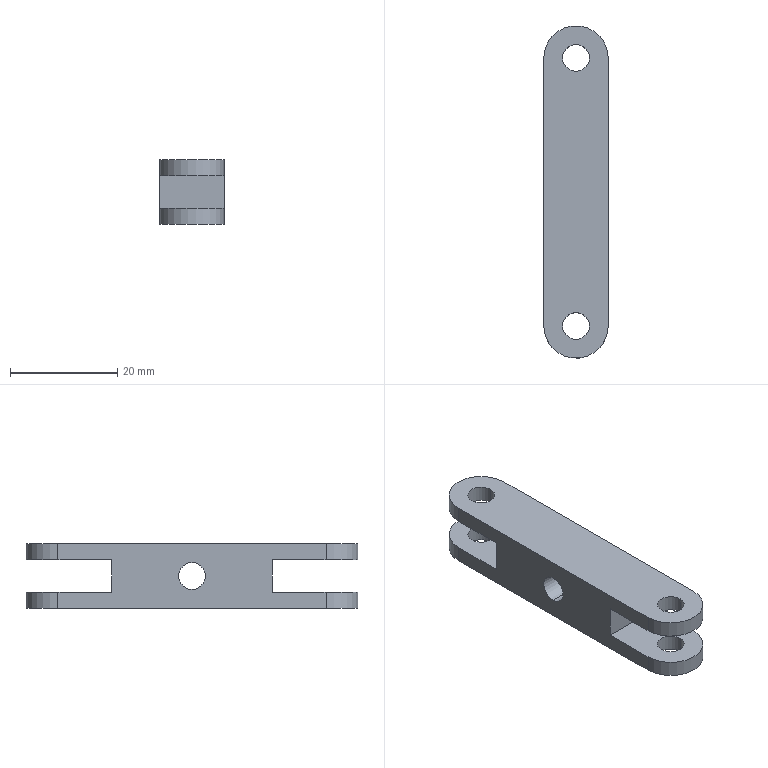Part | SolidWorks | features ICE 2, 3DProfileFeature 1, Extrusion 1, HoleWzd 1 | 1 solid | 24 faces | box 12 x 62 x 12 mm | volume 5967 mm3 | cylinder 14 | plane 10 | commonest cylinder face diameters 5 x10 12 x4
STEP:
#1=CARTESIAN_POINT('',(-6.,25.,8.5));
#2=VERTEX_POINT('',#1);
#3=CARTESIAN_POINT('',(-6.,25.,3.5));
#4=VERTEX_POINT('',#3);
#5=CARTESIAN_POINT('',(-6.,25.,6.));
#6=DIRECTION('',(1.,0.,0.));
#7=DIRECTION('',(0.,0.,-1.));
#8=AXIS2_PLACEMENT_3D('',#5,#6,#7);
#9=CIRCLE('',#8,2.5);
#10=EDGE_CURVE('',#2,#4,#9,.T.);
#11=ORIENTED_EDGE('',*,*,#10,.F.);
#12=CARTESIAN_POINT('',(6.,25.,8.5));
#13=VERTEX_POINT('',#12);
#14=CARTESIAN_POINT('',(6.,25.,8.5));
#15=DIRECTION('',(1.,0.,0.));
#16=VECTOR('',#15,1000.);
#17=LINE('',#14,#16);
#18=EDGE_CURVE('',#2,#13,#17,.T.);
#19=ORIENTED_EDGE('',*,*,#18,.T.);
#20=CARTESIAN_POINT('',(6.,25.,3.5));
#21=VERTEX_POINT('',#20);
#22=CARTESIAN_POINT('',(6.,25.,6.));
#23=DIRECTION('',(1.,0.,0.));
#24=DIRECTION('',(0.,0.,-1.));
#25=AXIS2_PLACEMENT_3D('',#22,#23,#24);
#26=CIRCLE('',#25,2.5);
#27=EDGE_CURVE('',#13,#21,#26,.T.);
#28=ORIENTED_EDGE('',*,*,#27,.T.);
#29=CARTESIAN_POINT('',(6.,25.,3.5));
#30=DIRECTION('',(1.,0.,0.));
#31=VECTOR('',#30,1000.);
#32=LINE('',#29,#31);
#33=EDGE_CURVE('',#4,#21,#32,.T.);
#34=ORIENTED_EDGE('',*,*,#33,.F.);
#35=EDGE_LOOP('',(#11,#19,#28,#34));
#36=FACE_OUTER_BOUND('',#35,.T.);
#37=CARTESIAN_POINT('',(6.,25.,6.));
#38=DIRECTION('',(1.,0.,0.));
#39=DIRECTION('',(0.,0.,-1.));
#40=AXIS2_PLACEMENT_3D('',#37,#38,#39);
#41=CYLINDRICAL_SURFACE('',#40,2.5);
#42=ADVANCED_FACE('',(#36),#41,.F.);
#43=CARTESIAN_POINT('',(-2.5,0.,0.));
#44=VERTEX_POINT('',#43);
#45=CARTESIAN_POINT('',(2.5,0.,0.));
#46=VERTEX_POINT('',#45);
#47=CARTESIAN_POINT('',(0.,0.,0.));
#48=DIRECTION('',(0.,0.,1.));
#49=DIRECTION('',(1.,0.,0.));
#50=AXIS2_PLACEMENT_3D('',#47,#48,#49);
#51=CIRCLE('',#50,2.5);
#52=EDGE_CURVE('',#44,#46,#51,.T.);
#53=ORIENTED_EDGE('',*,*,#52,.F.);
#54=CARTESIAN_POINT('',(-2.5,0.,3.));
#55=VERTEX_POINT('',#54);
#56=CARTESIAN_POINT('',(-2.5,0.,0.));
#57=DIRECTION('',(0.,0.,1.));
#58=VECTOR('',#57,1000.);
#59=LINE('',#56,#58);
#60=EDGE_CURVE('',#44,#55,#59,.T.);
#61=ORIENTED_EDGE('',*,*,#60,.T.);
#62=CARTESIAN_POINT('',(2.5,0.,3.));
#63=VERTEX_POINT('',#62);
#64=CARTESIAN_POINT('',(0.,0.,3.));
#65=DIRECTION('',(0.,0.,-1.));
#66=DIRECTION('',(-1.,0.,0.));
#67=AXIS2_PLACEMENT_3D('',#64,#65,#66);
#68=CIRCLE('',#67,2.5);
#69=EDGE_CURVE('',#63,#55,#68,.T.);
#70=ORIENTED_EDGE('',*,*,#69,.F.);
#71=CARTESIAN_POINT('',(2.5,0.,0.));
#72=DIRECTION('',(0.,0.,1.));
#73=VECTOR('',#72,1000.);
#74=LINE('',#71,#73);
#75=EDGE_CURVE('',#46,#63,#74,.T.);
#76=ORIENTED_EDGE('',*,*,#75,.F.);
#77=EDGE_LOOP('',(#53,#61,#70,#76));
#78=FACE_OUTER_BOUND('',#77,.T.);
#79=CARTESIAN_POINT('',(0.,0.,0.));
#80=DIRECTION('',(0.,0.,1.));
#81=DIRECTION('',(1.,0.,0.));
#82=AXIS2_PLACEMENT_3D('',#79,#80,#81);
#83=CYLINDRICAL_SURFACE('',#82,2.5);
#84=ADVANCED_FACE('',(#78),#83,.F.);
#85=CARTESIAN_POINT('',(-2.5,0.,9.));
#86=VERTEX_POINT('',#85);
#87=CARTESIAN_POINT('',(2.5,0.,9.));
#88=VERTEX_POINT('',#87);
#89=CARTESIAN_POINT('',(0.,0.,9.));
#90=DIRECTION('',(0.,0.,1.));
#91=DIRECTION('',(1.,0.,0.));
#92=AXIS2_PLACEMENT_3D('',#89,#90,#91);
#93=CIRCLE('',#92,2.5);
#94=EDGE_CURVE('',#86,#88,#93,.T.);
#95=ORIENTED_EDGE('',*,*,#94,.F.);
#96=CARTESIAN_POINT('',(-2.5,0.,12.));
#97=VERTEX_POINT('',#96);
#98=CARTESIAN_POINT('',(-2.5,0.,0.));
#99=DIRECTION('',(0.,0.,1.));
#100=VECTOR('',#99,1000.);
#101=LINE('',#98,#100);
#102=EDGE_CURVE('',#86,#97,#101,.T.);
#103=ORIENTED_EDGE('',*,*,#102,.T.);
#104=CARTESIAN_POINT('',(2.5,0.,12.));
#105=VERTEX_POINT('',#104);
#106=CARTESIAN_POINT('',(0.,0.,12.));
#107=DIRECTION('',(0.,0.,1.));
#108=DIRECTION('',(1.,0.,0.));
#109=AXIS2_PLACEMENT_3D('',#106,#107,#108);
#110=CIRCLE('',#109,2.5);
#111=EDGE_CURVE('',#97,#105,#110,.T.);
#112=ORIENTED_EDGE('',*,*,#111,.T.);
#113=CARTESIAN_POINT('',(2.5,0.,0.));
#114=DIRECTION('',(0.,0.,1.));
#115=VECTOR('',#114,1000.);
#116=LINE('',#113,#115);
#117=EDGE_CURVE('',#88,#105,#116,.T.);
#118=ORIENTED_EDGE('',*,*,#117,.F.);
#119=EDGE_LOOP('',(#95,#103,#112,#118));
#120=FACE_OUTER_BOUND('',#119,.T.);
#121=CARTESIAN_POINT('',(0.,0.,0.));
#122=DIRECTION('',(0.,0.,1.));
#123=DIRECTION('',(1.,0.,0.));
#124=AXIS2_PLACEMENT_3D('',#121,#122,#123);
#125=CYLINDRICAL_SURFACE('',#124,2.5);
#126=ADVANCED_FACE('',(#120),#125,.F.);
#127=CARTESIAN_POINT('',(-2.5,50.,9.));
#128=VERTEX_POINT('',#127);
#129=CARTESIAN_POINT('',(2.5,50.,9.));
#130=VERTEX_POINT('',#129);
#131=CARTESIAN_POINT('',(0.,50.,9.));
#132=DIRECTION('',(0.,0.,1.));
#133=DIRECTION('',(0.,-1.,0.));
#134=AXIS2_PLACEMENT_3D('',#131,#132,#133);
#135=CIRCLE('',#134,2.5);
#136=EDGE_CURVE('',#128,#130,#135,.T.);
#137=ORIENTED_EDGE('',*,*,#136,.F.);
#138=CARTESIAN_POINT('',(-2.5,50.,12.));
#139=VERTEX_POINT('',#138);
#140=CARTESIAN_POINT('',(-2.5,50.,0.));
#141=DIRECTION('',(0.,0.,1.));
#142=VECTOR('',#141,1000.);
#143=LINE('',#140,#142);
#144=EDGE_CURVE('',#128,#139,#143,.T.);
#145=ORIENTED_EDGE('',*,*,#144,.T.);
#146=CARTESIAN_POINT('',(2.5,50.,12.));
#147=VERTEX_POINT('',#146);
#148=CARTESIAN_POINT('',(0.,50.,12.));
#149=DIRECTION('',(0.,0.,1.));
#150=DIRECTION('',(1.,0.,0.));
#151=AXIS2_PLACEMENT_3D('',#148,#149,#150);
#152=CIRCLE('',#151,2.5);
#153=EDGE_CURVE('',#139,#147,#152,.T.);
#154=ORIENTED_EDGE('',*,*,#153,.T.);
#155=CARTESIAN_POINT('',(2.5,50.,0.));
#156=DIRECTION('',(0.,0.,1.));
#157=VECTOR('',#156,1000.);
#158=LINE('',#155,#157);
#159=EDGE_CURVE('',#130,#147,#158,.T.);
#160=ORIENTED_EDGE('',*,*,#159,.F.);
#161=EDGE_LOOP('',(#137,#145,#154,#160));
#162=FACE_OUTER_BOUND('',#161,.T.);
#163=CARTESIAN_POINT('',(0.,50.,0.));
#164=DIRECTION('',(0.,0.,1.));
#165=DIRECTION('',(1.,0.,0.));
#166=AXIS2_PLACEMENT_3D('',#163,#164,#165);
#167=CYLINDRICAL_SURFACE('',#166,2.5);
#168=ADVANCED_FACE('',(#162),#167,.F.);
#169=CARTESIAN_POINT('',(-2.5,50.,0.));
#170=VERTEX_POINT('',#169);
#171=CARTESIAN_POINT('',(2.5,50.,0.));
#172=VERTEX_POINT('',#171);
#173=CARTESIAN_POINT('',(0.,50.,0.));
#174=DIRECTION('',(0.,0.,1.));
#175=DIRECTION('',(1.,0.,0.));
#176=AXIS2_PLACEMENT_3D('',#173,#174,#175);
#177=CIRCLE('',#176,2.5);
#178=EDGE_CURVE('',#170,#172,#177,.T.);
#179=ORIENTED_EDGE('',*,*,#178,.F.);
#180=CARTESIAN_POINT('',(-2.5,50.,3.));
#181=VERTEX_POINT('',#180);
#182=CARTESIAN_POINT('',(-2.5,50.,0.));
#183=DIRECTION('',(0.,0.,1.));
#184=VECTOR('',#183,1000.);
#185=LINE('',#182,#184);
#186=EDGE_CURVE('',#170,#181,#185,.T.);
#187=ORIENTED_EDGE('',*,*,#186,.T.);
#188=CARTESIAN_POINT('',(2.5,50.,3.));
#189=VERTEX_POINT('',#188);
#190=CARTESIAN_POINT('',(0.,50.,3.));
#191=DIRECTION('',(0.,0.,-1.));
#192=DIRECTION('',(-1.,0.,0.));
#193=AXIS2_PLACEMENT_3D('',#190,#191,#192);
#194=CIRCLE('',#193,2.5);
#195=EDGE_CURVE('',#189,#181,#194,.T.);
#196=ORIENTED_EDGE('',*,*,#195,.F.);
#197=CARTESIAN_POINT('',(2.5,50.,0.));
#198=DIRECTION('',(0.,0.,1.));
#199=VECTOR('',#198,1000.);
#200=LINE('',#197,#199);
#201=EDGE_CURVE('',#172,#189,#200,.T.);
#202=ORIENTED_EDGE('',*,*,#201,.F.);
#203=EDGE_LOOP('',(#179,#187,#196,#202));
#204=FACE_OUTER_BOUND('',#203,.T.);
#205=CARTESIAN_POINT('',(0.,50.,0.));
#206=DIRECTION('',(0.,0.,1.));
#207=DIRECTION('',(1.,0.,0.));
#208=AXIS2_PLACEMENT_3D('',#205,#206,#207);
#209=CYLINDRICAL_SURFACE('',#208,2.5);
#210=ADVANCED_FACE('',(#204),#209,.F.);
#211=CARTESIAN_POINT('',(6.,0.,3.));
#212=VERTEX_POINT('',#211);
#213=CARTESIAN_POINT('',(6.,0.,0.));
#214=VERTEX_POINT('',#213);
#215=CARTESIAN_POINT('',(6.,0.,12.));
#216=DIRECTION('',(0.,0.,-1.));
#217=VECTOR('',#216,1000.);
#218=LINE('',#215,#217);
#219=EDGE_CURVE('',#212,#214,#218,.T.);
#220=ORIENTED_EDGE('',*,*,#219,.F.);
#221=CARTESIAN_POINT('',(-6.,0.,3.));
#222=VERTEX_POINT('',#221);
#223=CARTESIAN_POINT('',(0.,0.,3.));
#224=DIRECTION('',(0.,0.,-1.));
#225=DIRECTION('',(-1.,0.,0.));
#226=AXIS2_PLACEMENT_3D('',#223,#224,#225);
#227=CIRCLE('',#226,6.);
#228=EDGE_CURVE('',#212,#222,#227,.T.);
#229=ORIENTED_EDGE('',*,*,#228,.T.);
#230=CARTESIAN_POINT('',(-6.,0.,0.));
#231=VERTEX_POINT('',#230);
#232=CARTESIAN_POINT('',(-6.,0.,12.));
#233=DIRECTION('',(0.,0.,-1.));
#234=VECTOR('',#233,1000.);
#235=LINE('',#232,#234);
#236=EDGE_CURVE('',#222,#231,#235,.T.);
#237=ORIENTED_EDGE('',*,*,#236,.T.);
#238=CARTESIAN_POINT('',(0.,0.,0.));
#239=DIRECTION('',(0.,0.,1.));
#240=DIRECTION('',(1.,0.,0.));
#241=AXIS2_PLACEMENT_3D('',#238,#239,#240);
#242=CIRCLE('',#241,6.);
#243=EDGE_CURVE('',#231,#214,#242,.T.);
#244=ORIENTED_EDGE('',*,*,#243,.T.);
#245=EDGE_LOOP('',(#220,#229,#237,#244));
#246=FACE_OUTER_BOUND('',#245,.T.);
#247=CARTESIAN_POINT('',(0.,0.,12.));
#248=DIRECTION('',(0.,0.,-1.));
#249=DIRECTION('',(-1.,0.,0.));
#250=AXIS2_PLACEMENT_3D('',#247,#248,#249);
#251=CYLINDRICAL_SURFACE('',#250,6.);
#252=ADVANCED_FACE('',(#246),#251,.T.);
#253=CARTESIAN_POINT('',(6.,50.,12.));
#254=VERTEX_POINT('',#253);
#255=CARTESIAN_POINT('',(6.,50.,9.));
#256=VERTEX_POINT('',#255);
#257=CARTESIAN_POINT('',(6.,50.,12.));
#258=DIRECTION('',(0.,0.,-1.));
#259=VECTOR('',#258,1000.);
#260=LINE('',#257,#259);
#261=EDGE_CURVE('',#254,#256,#260,.T.);
#262=ORIENTED_EDGE('',*,*,#261,.T.);
#263=CARTESIAN_POINT('',(-6.,50.,9.));
#264=VERTEX_POINT('',#263);
#265=CARTESIAN_POINT('',(0.,50.,9.));
#266=DIRECTION('',(0.,0.,1.));
#267=DIRECTION('',(0.,-1.,0.));
#268=AXIS2_PLACEMENT_3D('',#265,#266,#267);
#269=CIRCLE('',#268,6.);
#270=EDGE_CURVE('',#256,#264,#269,.T.);
#271=ORIENTED_EDGE('',*,*,#270,.T.);
#272=CARTESIAN_POINT('',(-6.,50.,12.));
#273=VERTEX_POINT('',#272);
#274=CARTESIAN_POINT('',(-6.,50.,12.));
#275=DIRECTION('',(0.,0.,-1.));
#276=VECTOR('',#275,1000.);
#277=LINE('',#274,#276);
#278=EDGE_CURVE('',#273,#264,#277,.T.);
#279=ORIENTED_EDGE('',*,*,#278,.F.);
#280=CARTESIAN_POINT('',(0.,50.,12.));
#281=DIRECTION('',(0.,0.,1.));
#282=DIRECTION('',(1.,0.,0.));
#283=AXIS2_PLACEMENT_3D('',#280,#281,#282);
#284=CIRCLE('',#283,6.);
#285=EDGE_CURVE('',#254,#273,#284,.T.);
#286=ORIENTED_EDGE('',*,*,#285,.F.);
#287=EDGE_LOOP('',(#262,#271,#279,#286));
#288=FACE_OUTER_BOUND('',#287,.T.);
#289=CARTESIAN_POINT('',(0.,50.,12.));
#290=DIRECTION('',(0.,0.,-1.));
#291=DIRECTION('',(-1.,0.,0.));
#292=AXIS2_PLACEMENT_3D('',#289,#290,#291);
#293=CYLINDRICAL_SURFACE('',#292,6.);
#294=ADVANCED_FACE('',(#288),#293,.T.);
#295=CARTESIAN_POINT('',(-6.,0.,12.));
#296=VERTEX_POINT('',#295);
#297=CARTESIAN_POINT('',(-6.,0.,9.));
#298=VERTEX_POINT('',#297);
#299=CARTESIAN_POINT('',(-6.,0.,12.));
#300=DIRECTION('',(0.,0.,-1.));
#301=VECTOR('',#300,1000.);
#302=LINE('',#299,#301);
#303=EDGE_CURVE('',#296,#298,#302,.T.);
#304=ORIENTED_EDGE('',*,*,#303,.T.);
#305=CARTESIAN_POINT('',(6.,0.,9.));
#306=VERTEX_POINT('',#305);
#307=CARTESIAN_POINT('',(0.,0.,9.));
#308=DIRECTION('',(0.,0.,1.));
#309=DIRECTION('',(1.,0.,0.));
#310=AXIS2_PLACEMENT_3D('',#307,#308,#309);
#311=CIRCLE('',#310,6.);
#312=EDGE_CURVE('',#298,#306,#311,.T.);
#313=ORIENTED_EDGE('',*,*,#312,.T.);
#314=CARTESIAN_POINT('',(6.,0.,12.));
#315=VERTEX_POINT('',#314);
#316=CARTESIAN_POINT('',(6.,0.,12.));
#317=DIRECTION('',(0.,0.,-1.));
#318=VECTOR('',#317,1000.);
#319=LINE('',#316,#318);
#320=EDGE_CURVE('',#315,#306,#319,.T.);
#321=ORIENTED_EDGE('',*,*,#320,.F.);
#322=CARTESIAN_POINT('',(0.,0.,12.));
#323=DIRECTION('',(0.,0.,1.));
#324=DIRECTION('',(1.,0.,0.));
#325=AXIS2_PLACEMENT_3D('',#322,#323,#324);
#326=CIRCLE('',#325,6.);
#327=EDGE_CURVE('',#296,#315,#326,.T.);
#328=ORIENTED_EDGE('',*,*,#327,.F.);
#329=EDGE_LOOP('',(#304,#313,#321,#328));
#330=FACE_OUTER_BOUND('',#329,.T.);
#331=CARTESIAN_POINT('',(0.,0.,12.));
#332=DIRECTION('',(0.,0.,-1.));
#333=DIRECTION('',(-1.,0.,0.));
#334=AXIS2_PLACEMENT_3D('',#331,#332,#333);
#335=CYLINDRICAL_SURFACE('',#334,6.);
#336=ADVANCED_FACE('',(#330),#335,.T.);
#337=CARTESIAN_POINT('',(6.,25.,6.));
#338=DIRECTION('',(1.,0.,0.));
#339=DIRECTION('',(0.,0.,-1.));
#340=AXIS2_PLACEMENT_3D('',#337,#338,#339);
#341=CIRCLE('',#340,2.5);
#342=EDGE_CURVE('',#21,#13,#341,.T.);
#343=ORIENTED_EDGE('',*,*,#342,.F.);
#344=ORIENTED_EDGE('',*,*,#27,.F.);
#345=EDGE_LOOP('',(#343,#344));
#346=FACE_BOUND('',#345,.T.);
#347=CARTESIAN_POINT('',(6.,40.,3.));
#348=VERTEX_POINT('',#347);
#349=CARTESIAN_POINT('',(6.,40.,9.));
#350=VERTEX_POINT('',#349);
#351=CARTESIAN_POINT('',(6.,40.,3.));
#352=DIRECTION('',(0.,0.,1.));
#353=VECTOR('',#352,1000.);
#354=LINE('',#351,#353);
#355=EDGE_CURVE('',#348,#350,#354,.T.);
#356=ORIENTED_EDGE('',*,*,#355,.T.);
#357=CARTESIAN_POINT('',(6.,72.,9.));
#358=DIRECTION('',(0.,1.,0.));
#359=VECTOR('',#358,1000.);
#360=LINE('',#357,#359);
#361=EDGE_CURVE('',#350,#256,#360,.T.);
#362=ORIENTED_EDGE('',*,*,#361,.T.);
#363=ORIENTED_EDGE('',*,*,#261,.F.);
#364=CARTESIAN_POINT('',(6.,0.,12.));
#365=DIRECTION('',(0.,1.,0.));
#366=VECTOR('',#365,1000.);
#367=LINE('',#364,#366);
#368=EDGE_CURVE('',#315,#254,#367,.T.);
#369=ORIENTED_EDGE('',*,*,#368,.F.);
#370=ORIENTED_EDGE('',*,*,#320,.T.);
#371=CARTESIAN_POINT('',(6.,10.,9.));
#372=VERTEX_POINT('',#371);
#373=CARTESIAN_POINT('',(6.,-22.,9.));
#374=DIRECTION('',(0.,1.,0.));
#375=VECTOR('',#374,1000.);
#376=LINE('',#373,#375);
#377=EDGE_CURVE('',#306,#372,#376,.T.);
#378=ORIENTED_EDGE('',*,*,#377,.T.);
#379=CARTESIAN_POINT('',(6.,10.,3.));
#380=VERTEX_POINT('',#379);
#381=CARTESIAN_POINT('',(6.,10.,3.));
#382=DIRECTION('',(0.,0.,-1.));
#383=VECTOR('',#382,1000.);
#384=LINE('',#381,#383);
#385=EDGE_CURVE('',#372,#380,#384,.T.);
#386=ORIENTED_EDGE('',*,*,#385,.T.);
#387=CARTESIAN_POINT('',(6.,-22.,3.));
#388=DIRECTION('',(0.,-1.,0.));
#389=VECTOR('',#388,1000.);
#390=LINE('',#387,#389);
#391=EDGE_CURVE('',#380,#212,#390,.T.);
#392=ORIENTED_EDGE('',*,*,#391,.T.);
#393=ORIENTED_EDGE('',*,*,#219,.T.);
#394=CARTESIAN_POINT('',(6.,50.,0.));
#395=VERTEX_POINT('',#394);
#396=CARTESIAN_POINT('',(6.,0.,0.));
#397=DIRECTION('',(0.,1.,0.));
#398=VECTOR('',#397,1000.);
#399=LINE('',#396,#398);
#400=EDGE_CURVE('',#214,#395,#399,.T.);
#401=ORIENTED_EDGE('',*,*,#400,.T.);
#402=CARTESIAN_POINT('',(6.,50.,3.));
#403=VERTEX_POINT('',#402);
#404=CARTESIAN_POINT('',(6.,50.,12.));
#405=DIRECTION('',(0.,0.,-1.));
#406=VECTOR('',#405,1000.);
#407=LINE('',#404,#406);
#408=EDGE_CURVE('',#403,#395,#407,.T.);
#409=ORIENTED_EDGE('',*,*,#408,.F.);
#410=CARTESIAN_POINT('',(6.,72.,3.));
#411=DIRECTION('',(0.,-1.,0.));
#412=VECTOR('',#411,1000.);
#413=LINE('',#410,#412);
#414=EDGE_CURVE('',#403,#348,#413,.T.);
#415=ORIENTED_EDGE('',*,*,#414,.T.);
#416=EDGE_LOOP('',(#356,#362,#363,#369,#370,#378,#386,#392,#393,#401,#409,#415));
#417=FACE_OUTER_BOUND('',#416,.T.);
#418=CARTESIAN_POINT('',(6.,0.,12.));
#419=DIRECTION('',(-1.,0.,0.));
#420=DIRECTION('',(0.,0.,1.));
#421=AXIS2_PLACEMENT_3D('',#418,#419,#420);
#422=PLANE('',#421);
#423=ADVANCED_FACE('',(#346,#417),#422,.F.);
#424=CARTESIAN_POINT('',(-6.,50.,3.));
#425=VERTEX_POINT('',#424);
#426=CARTESIAN_POINT('',(-6.,50.,0.));
#427=VERTEX_POINT('',#426);
#428=CARTESIAN_POINT('',(-6.,50.,12.));
#429=DIRECTION('',(0.,0.,-1.));
#430=VECTOR('',#429,1000.);
#431=LINE('',#428,#430);
#432=EDGE_CURVE('',#425,#427,#431,.T.);
#433=ORIENTED_EDGE('',*,*,#432,.F.);
#434=CARTESIAN_POINT('',(0.,50.,3.));
#435=DIRECTION('',(0.,0.,-1.));
#436=DIRECTION('',(-1.,0.,0.));
#437=AXIS2_PLACEMENT_3D('',#434,#435,#436);
#438=CIRCLE('',#437,6.);
#439=EDGE_CURVE('',#425,#403,#438,.T.);
#440=ORIENTED_EDGE('',*,*,#439,.T.);
#441=ORIENTED_EDGE('',*,*,#408,.T.);
#442=CARTESIAN_POINT('',(0.,50.,0.));
#443=DIRECTION('',(0.,0.,1.));
#444=DIRECTION('',(1.,0.,0.));
#445=AXIS2_PLACEMENT_3D('',#442,#443,#444);
#446=CIRCLE('',#445,6.);
#447=EDGE_CURVE('',#395,#427,#446,.T.);
#448=ORIENTED_EDGE('',*,*,#447,.T.);
#449=EDGE_LOOP('',(#433,#440,#441,#448));
#450=FACE_OUTER_BOUND('',#449,.T.);
#451=CARTESIAN_POINT('',(0.,50.,12.));
#452=DIRECTION('',(0.,0.,-1.));
#453=DIRECTION('',(-1.,0.,0.));
#454=AXIS2_PLACEMENT_3D('',#451,#452,#453);
#455=CYLINDRICAL_SURFACE('',#454,6.);
#456=ADVANCED_FACE('',(#450),#455,.T.);
#457=CARTESIAN_POINT('',(-6.,25.,6.));
#458=DIRECTION('',(1.,0.,0.));
#459=DIRECTION('',(0.,0.,-1.));
#460=AXIS2_PLACEMENT_3D('',#457,#458,#459);
#461=CIRCLE('',#460,2.5);
#462=EDGE_CURVE('',#4,#2,#461,.T.);
#463=ORIENTED_EDGE('',*,*,#462,.T.);
#464=ORIENTED_EDGE('',*,*,#10,.T.);
#465=EDGE_LOOP('',(#463,#464));
#466=FACE_BOUND('',#465,.T.);
#467=ORIENTED_EDGE('',*,*,#278,.T.);
#468=CARTESIAN_POINT('',(-6.,40.,9.));
#469=VERTEX_POINT('',#468);
#470=CARTESIAN_POINT('',(-6.,72.,9.));
#471=DIRECTION('',(0.,1.,0.));
#472=VECTOR('',#471,1000.);
#473=LINE('',#470,#472);
#474=EDGE_CURVE('',#469,#264,#473,.T.);
#475=ORIENTED_EDGE('',*,*,#474,.F.);
#476=CARTESIAN_POINT('',(-6.,40.,3.));
#477=VERTEX_POINT('',#476);
#478=CARTESIAN_POINT('',(-6.,40.,3.));
#479=DIRECTION('',(0.,0.,1.));
#480=VECTOR('',#479,1000.);
#481=LINE('',#478,#480);
#482=EDGE_CURVE('',#477,#469,#481,.T.);
#483=ORIENTED_EDGE('',*,*,#482,.F.);
#484=CARTESIAN_POINT('',(-6.,0.,3.));
#485=DIRECTION('',(0.,1.,0.));
#486=VECTOR('',#485,1000.);
#487=LINE('',#484,#486);
#488=EDGE_CURVE('',#477,#425,#487,.T.);
#489=ORIENTED_EDGE('',*,*,#488,.T.);
#490=ORIENTED_EDGE('',*,*,#432,.T.);
#491=CARTESIAN_POINT('',(-6.,0.,0.));
#492=DIRECTION('',(0.,-1.,0.));
#493=VECTOR('',#492,1000.);
#494=LINE('',#491,#493);
#495=EDGE_CURVE('',#427,#231,#494,.T.);
#496=ORIENTED_EDGE('',*,*,#495,.T.);
#497=ORIENTED_EDGE('',*,*,#236,.F.);
#498=CARTESIAN_POINT('',(-6.,10.,3.));
#499=VERTEX_POINT('',#498);
#500=CARTESIAN_POINT('',(-6.,-22.,3.));
#501=DIRECTION('',(0.,-1.,0.));
#502=VECTOR('',#501,1000.);
#503=LINE('',#500,#502);
#504=EDGE_CURVE('',#499,#222,#503,.T.);
#505=ORIENTED_EDGE('',*,*,#504,.F.);
#506=CARTESIAN_POINT('',(-6.,10.,9.));
#507=VERTEX_POINT('',#506);
#508=CARTESIAN_POINT('',(-6.,10.,3.));
#509=DIRECTION('',(0.,0.,-1.));
#510=VECTOR('',#509,1000.);
#511=LINE('',#508,#510);
#512=EDGE_CURVE('',#507,#499,#511,.T.);
#513=ORIENTED_EDGE('',*,*,#512,.F.);
#514=CARTESIAN_POINT('',(-6.,0.,9.));
#515=DIRECTION('',(0.,-1.,0.));
#516=VECTOR('',#515,1000.);
#517=LINE('',#514,#516);
#518=EDGE_CURVE('',#507,#298,#517,.T.);
#519=ORIENTED_EDGE('',*,*,#518,.T.);
#520=ORIENTED_EDGE('',*,*,#303,.F.);
#521=CARTESIAN_POINT('',(-6.,0.,12.));
#522=DIRECTION('',(0.,-1.,0.));
#523=VECTOR('',#522,1000.);
#524=LINE('',#521,#523);
#525=EDGE_CURVE('',#273,#296,#524,.T.);
#526=ORIENTED_EDGE('',*,*,#525,.F.);
#527=EDGE_LOOP('',(#467,#475,#483,#489,#490,#496,#497,#505,#513,#519,#520,#526));
#528=FACE_OUTER_BOUND('',#527,.T.);
#529=CARTESIAN_POINT('',(-6.,0.,12.));
#530=DIRECTION('',(1.,0.,0.));
#531=DIRECTION('',(0.,0.,-1.));
#532=AXIS2_PLACEMENT_3D('',#529,#530,#531);
#533=PLANE('',#532);
#534=ADVANCED_FACE('',(#466,#528),#533,.F.);
#535=CARTESIAN_POINT('',(0.,50.,12.));
#536=DIRECTION('',(0.,0.,1.));
#537=DIRECTION('',(1.,0.,0.));
#538=AXIS2_PLACEMENT_3D('',#535,#536,#537);
#539=CIRCLE('',#538,2.5);
#540=EDGE_CURVE('',#147,#139,#539,.T.);
#541=ORIENTED_EDGE('',*,*,#540,.F.);
#542=ORIENTED_EDGE('',*,*,#153,.F.);
#543=EDGE_LOOP('',(#541,#542));
#544=FACE_BOUND('',#543,.T.);
#545=CARTESIAN_POINT('',(0.,0.,12.));
#546=DIRECTION('',(0.,0.,1.));
#547=DIRECTION('',(1.,0.,0.));
#548=AXIS2_PLACEMENT_3D('',#545,#546,#547);
#549=CIRCLE('',#548,2.5);
#550=EDGE_CURVE('',#105,#97,#549,.T.);
#551=ORIENTED_EDGE('',*,*,#550,.F.);
#552=ORIENTED_EDGE('',*,*,#111,.F.);
#553=EDGE_LOOP('',(#551,#552));
#554=FACE_BOUND('',#553,.T.);
#555=ORIENTED_EDGE('',*,*,#327,.T.);
#556=ORIENTED_EDGE('',*,*,#368,.T.);
#557=ORIENTED_EDGE('',*,*,#285,.T.);
#558=ORIENTED_EDGE('',*,*,#525,.T.);
#559=EDGE_LOOP('',(#555,#556,#557,#558));
#560=FACE_OUTER_BOUND('',#559,.T.);
#561=CARTESIAN_POINT('',(0.,0.,12.));
#562=DIRECTION('',(0.,0.,1.));
#563=DIRECTION('',(1.,0.,0.));
#564=AXIS2_PLACEMENT_3D('',#561,#562,#563);
#565=PLANE('',#564);
#566=ADVANCED_FACE('',(#544,#554,#560),#565,.T.);
#567=CARTESIAN_POINT('',(0.,50.,0.));
#568=DIRECTION('',(0.,0.,1.));
#569=DIRECTION('',(1.,0.,0.));
#570=AXIS2_PLACEMENT_3D('',#567,#568,#569);
#571=CIRCLE('',#570,2.5);
#572=EDGE_CURVE('',#172,#170,#571,.T.);
#573=ORIENTED_EDGE('',*,*,#572,.T.);
#574=ORIENTED_EDGE('',*,*,#178,.T.);
#575=EDGE_LOOP('',(#573,#574));
#576=FACE_BOUND('',#575,.T.);
#577=CARTESIAN_POINT('',(0.,0.,0.));
#578=DIRECTION('',(0.,0.,1.));
#579=DIRECTION('',(1.,0.,0.));
#580=AXIS2_PLACEMENT_3D('',#577,#578,#579);
#581=CIRCLE('',#580,2.5);
#582=EDGE_CURVE('',#46,#44,#581,.T.);
#583=ORIENTED_EDGE('',*,*,#582,.T.);
#584=ORIENTED_EDGE('',*,*,#52,.T.);
#585=EDGE_LOOP('',(#583,#584));
#586=FACE_BOUND('',#585,.T.);
#587=ORIENTED_EDGE('',*,*,#243,.F.);
#588=ORIENTED_EDGE('',*,*,#495,.F.);
#589=ORIENTED_EDGE('',*,*,#447,.F.);
#590=ORIENTED_EDGE('',*,*,#400,.F.);
#591=EDGE_LOOP('',(#587,#588,#589,#590));
#592=FACE_OUTER_BOUND('',#591,.T.);
#593=CARTESIAN_POINT('',(0.,0.,0.));
#594=DIRECTION('',(0.,0.,1.));
#595=DIRECTION('',(1.,0.,0.));
#596=AXIS2_PLACEMENT_3D('',#593,#594,#595);
#597=PLANE('',#596);
#598=ADVANCED_FACE('',(#576,#586,#592),#597,.F.);
#599=ORIENTED_EDGE('',*,*,#69,.T.);
#600=CARTESIAN_POINT('',(0.,0.,3.));
#601=DIRECTION('',(0.,0.,-1.));
#602=DIRECTION('',(-1.,0.,0.));
#603=AXIS2_PLACEMENT_3D('',#600,#601,#602);
#604=CIRCLE('',#603,2.5);
#605=EDGE_CURVE('',#55,#63,#604,.T.);
#606=ORIENTED_EDGE('',*,*,#605,.T.);
#607=EDGE_LOOP('',(#599,#606));
#608=FACE_BOUND('',#607,.T.);
#609=ORIENTED_EDGE('',*,*,#391,.F.);
#610=CARTESIAN_POINT('',(6.,10.,3.));
#611=DIRECTION('',(-1.,0.,0.));
#612=VECTOR('',#611,1000.);
#613=LINE('',#610,#612);
#614=EDGE_CURVE('',#380,#499,#613,.T.);
#615=ORIENTED_EDGE('',*,*,#614,.T.);
#616=ORIENTED_EDGE('',*,*,#504,.T.);
#617=ORIENTED_EDGE('',*,*,#228,.F.);
#618=EDGE_LOOP('',(#609,#615,#616,#617));
#619=FACE_OUTER_BOUND('',#618,.T.);
#620=CARTESIAN_POINT('',(6.,-22.,3.));
#621=DIRECTION('',(0.,0.,-1.));
#622=DIRECTION('',(-1.,0.,0.));
#623=AXIS2_PLACEMENT_3D('',#620,#621,#622);
#624=PLANE('',#623);
#625=ADVANCED_FACE('',(#608,#619),#624,.F.);
#626=CARTESIAN_POINT('',(0.,0.,9.));
#627=DIRECTION('',(0.,0.,1.));
#628=DIRECTION('',(1.,0.,0.));
#629=AXIS2_PLACEMENT_3D('',#626,#627,#628);
#630=CIRCLE('',#629,2.5);
#631=EDGE_CURVE('',#88,#86,#630,.T.);
#632=ORIENTED_EDGE('',*,*,#631,.T.);
#633=ORIENTED_EDGE('',*,*,#94,.T.);
#634=EDGE_LOOP('',(#632,#633));
#635=FACE_BOUND('',#634,.T.);
#636=ORIENTED_EDGE('',*,*,#518,.F.);
#637=CARTESIAN_POINT('',(6.,10.,9.));
#638=DIRECTION('',(-1.,0.,0.));
#639=VECTOR('',#638,1000.);
#640=LINE('',#637,#639);
#641=EDGE_CURVE('',#372,#507,#640,.T.);
#642=ORIENTED_EDGE('',*,*,#641,.F.);
#643=ORIENTED_EDGE('',*,*,#377,.F.);
#644=ORIENTED_EDGE('',*,*,#312,.F.);
#645=EDGE_LOOP('',(#636,#642,#643,#644));
#646=FACE_OUTER_BOUND('',#645,.T.);
#647=CARTESIAN_POINT('',(6.,-22.,9.));
#648=DIRECTION('',(0.,0.,1.));
#649=DIRECTION('',(1.,0.,0.));
#650=AXIS2_PLACEMENT_3D('',#647,#648,#649);
#651=PLANE('',#650);
#652=ADVANCED_FACE('',(#635,#646),#651,.F.);
#653=ORIENTED_EDGE('',*,*,#512,.T.);
#654=ORIENTED_EDGE('',*,*,#614,.F.);
#655=ORIENTED_EDGE('',*,*,#385,.F.);
#656=ORIENTED_EDGE('',*,*,#641,.T.);
#657=EDGE_LOOP('',(#653,#654,#655,#656));
#658=FACE_OUTER_BOUND('',#657,.T.);
#659=CARTESIAN_POINT('',(6.,10.,3.));
#660=DIRECTION('',(0.,1.,0.));
#661=DIRECTION('',(-1.,0.,0.));
#662=AXIS2_PLACEMENT_3D('',#659,#660,#661);
#663=PLANE('',#662);
#664=ADVANCED_FACE('',(#658),#663,.F.);
#665=CARTESIAN_POINT('',(0.,50.,9.));
#666=DIRECTION('',(0.,0.,1.));
#667=DIRECTION('',(0.,-1.,0.));
#668=AXIS2_PLACEMENT_3D('',#665,#666,#667);
#669=CIRCLE('',#668,2.5);
#670=EDGE_CURVE('',#130,#128,#669,.T.);
#671=ORIENTED_EDGE('',*,*,#670,.T.);
#672=ORIENTED_EDGE('',*,*,#136,.T.);
#673=EDGE_LOOP('',(#671,#672));
#674=FACE_BOUND('',#673,.T.);
#675=ORIENTED_EDGE('',*,*,#361,.F.);
#676=CARTESIAN_POINT('',(6.,40.,9.));
#677=DIRECTION('',(-1.,0.,0.));
#678=VECTOR('',#677,1000.);
#679=LINE('',#676,#678);
#680=EDGE_CURVE('',#350,#469,#679,.T.);
#681=ORIENTED_EDGE('',*,*,#680,.T.);
#682=ORIENTED_EDGE('',*,*,#474,.T.);
#683=ORIENTED_EDGE('',*,*,#270,.F.);
#684=EDGE_LOOP('',(#675,#681,#682,#683));
#685=FACE_OUTER_BOUND('',#684,.T.);
#686=CARTESIAN_POINT('',(6.,72.,9.));
#687=DIRECTION('',(0.,0.,1.));
#688=DIRECTION('',(0.,-1.,0.));
#689=AXIS2_PLACEMENT_3D('',#686,#687,#688);
#690=PLANE('',#689);
#691=ADVANCED_FACE('',(#674,#685),#690,.F.);
#692=ORIENTED_EDGE('',*,*,#195,.T.);
#693=CARTESIAN_POINT('',(0.,50.,3.));
#694=DIRECTION('',(0.,0.,-1.));
#695=DIRECTION('',(-1.,0.,0.));
#696=AXIS2_PLACEMENT_3D('',#693,#694,#695);
#697=CIRCLE('',#696,2.5);
#698=EDGE_CURVE('',#181,#189,#697,.T.);
#699=ORIENTED_EDGE('',*,*,#698,.T.);
#700=EDGE_LOOP('',(#692,#699));
#701=FACE_BOUND('',#700,.T.);
#702=ORIENTED_EDGE('',*,*,#488,.F.);
#703=CARTESIAN_POINT('',(6.,40.,3.));
#704=DIRECTION('',(-1.,0.,0.));
#705=VECTOR('',#704,1000.);
#706=LINE('',#703,#705);
#707=EDGE_CURVE('',#348,#477,#706,.T.);
#708=ORIENTED_EDGE('',*,*,#707,.F.);
#709=ORIENTED_EDGE('',*,*,#414,.F.);
#710=ORIENTED_EDGE('',*,*,#439,.F.);
#711=EDGE_LOOP('',(#702,#708,#709,#710));
#712=FACE_OUTER_BOUND('',#711,.T.);
#713=CARTESIAN_POINT('',(6.,72.,3.));
#714=DIRECTION('',(0.,0.,-1.));
#715=DIRECTION('',(-1.,0.,0.));
#716=AXIS2_PLACEMENT_3D('',#713,#714,#715);
#717=PLANE('',#716);
#718=ADVANCED_FACE('',(#701,#712),#717,.F.);
#719=ORIENTED_EDGE('',*,*,#482,.T.);
#720=ORIENTED_EDGE('',*,*,#680,.F.);
#721=ORIENTED_EDGE('',*,*,#355,.F.);
#722=ORIENTED_EDGE('',*,*,#707,.T.);
#723=EDGE_LOOP('',(#719,#720,#721,#722));
#724=FACE_OUTER_BOUND('',#723,.T.);
#725=CARTESIAN_POINT('',(6.,40.,3.));
#726=DIRECTION('',(0.,-1.,0.));
#727=DIRECTION('',(1.,0.,0.));
#728=AXIS2_PLACEMENT_3D('',#725,#726,#727);
#729=PLANE('',#728);
#730=ADVANCED_FACE('',(#724),#729,.F.);
#731=ORIENTED_EDGE('',*,*,#186,.F.);
#732=ORIENTED_EDGE('',*,*,#572,.F.);
#733=ORIENTED_EDGE('',*,*,#201,.T.);
#734=ORIENTED_EDGE('',*,*,#698,.F.);
#735=EDGE_LOOP('',(#731,#732,#733,#734));
#736=FACE_OUTER_BOUND('',#735,.T.);
#737=CARTESIAN_POINT('',(0.,50.,0.));
#738=DIRECTION('',(0.,0.,1.));
#739=DIRECTION('',(1.,0.,0.));
#740=AXIS2_PLACEMENT_3D('',#737,#738,#739);
#741=CYLINDRICAL_SURFACE('',#740,2.5);
#742=ADVANCED_FACE('',(#736),#741,.F.);
#743=ORIENTED_EDGE('',*,*,#144,.F.);
#744=ORIENTED_EDGE('',*,*,#670,.F.);
#745=ORIENTED_EDGE('',*,*,#159,.T.);
#746=ORIENTED_EDGE('',*,*,#540,.T.);
#747=EDGE_LOOP('',(#743,#744,#745,#746));
#748=FACE_OUTER_BOUND('',#747,.T.);
#749=CARTESIAN_POINT('',(0.,50.,0.));
#750=DIRECTION('',(0.,0.,1.));
#751=DIRECTION('',(1.,0.,0.));
#752=AXIS2_PLACEMENT_3D('',#749,#750,#751);
#753=CYLINDRICAL_SURFACE('',#752,2.5);
#754=ADVANCED_FACE('',(#748),#753,.F.);
#755=ORIENTED_EDGE('',*,*,#102,.F.);
#756=ORIENTED_EDGE('',*,*,#631,.F.);
#757=ORIENTED_EDGE('',*,*,#117,.T.);
#758=ORIENTED_EDGE('',*,*,#550,.T.);
#759=EDGE_LOOP('',(#755,#756,#757,#758));
#760=FACE_OUTER_BOUND('',#759,.T.);
#761=CARTESIAN_POINT('',(0.,0.,0.));
#762=DIRECTION('',(0.,0.,1.));
#763=DIRECTION('',(1.,0.,0.));
#764=AXIS2_PLACEMENT_3D('',#761,#762,#763);
#765=CYLINDRICAL_SURFACE('',#764,2.5);
#766=ADVANCED_FACE('',(#760),#765,.F.);
#767=ORIENTED_EDGE('',*,*,#60,.F.);
#768=ORIENTED_EDGE('',*,*,#582,.F.);
#769=ORIENTED_EDGE('',*,*,#75,.T.);
#770=ORIENTED_EDGE('',*,*,#605,.F.);
#771=EDGE_LOOP('',(#767,#768,#769,#770));
#772=FACE_OUTER_BOUND('',#771,.T.);
#773=CARTESIAN_POINT('',(0.,0.,0.));
#774=DIRECTION('',(0.,0.,1.));
#775=DIRECTION('',(1.,0.,0.));
#776=AXIS2_PLACEMENT_3D('',#773,#774,#775);
#777=CYLINDRICAL_SURFACE('',#776,2.5);
#778=ADVANCED_FACE('',(#772),#777,.F.);
#779=ORIENTED_EDGE('',*,*,#18,.F.);
#780=ORIENTED_EDGE('',*,*,#462,.F.);
#781=ORIENTED_EDGE('',*,*,#33,.T.);
#782=ORIENTED_EDGE('',*,*,#342,.T.);
#783=EDGE_LOOP('',(#779,#780,#781,#782));
#784=FACE_OUTER_BOUND('',#783,.T.);
#785=CARTESIAN_POINT('',(6.,25.,6.));
#786=DIRECTION('',(1.,0.,0.));
#787=DIRECTION('',(0.,0.,-1.));
#788=AXIS2_PLACEMENT_3D('',#785,#786,#787);
#789=CYLINDRICAL_SURFACE('',#788,2.5);
#790=ADVANCED_FACE('',(#784),#789,.F.);
#791=CLOSED_SHELL('',(#42,#84,#126,#168,#210,#252,#294,#336,#423,#456,#534,#566,#598,#625,#652,#664,#691,#718,#730,#742,#754,#766,#778,#790));
#792=MANIFOLD_SOLID_BREP('',#791);
#793=CARTESIAN_POINT('',(0.,0.,0.));
#794=DIRECTION('',(0.,0.,1.));
#795=DIRECTION('',(1.,0.,0.));
#796=AXIS2_PLACEMENT_3D('',#793,#794,#795);
#797=(LENGTH_UNIT()NAMED_UNIT(*)SI_UNIT(.MILLI.,.METRE.));
#798=UNCERTAINTY_MEASURE_WITH_UNIT(LENGTH_MEASURE(0.00001),#797,'','');
#799=(NAMED_UNIT(*)PLANE_ANGLE_UNIT()SI_UNIT($,.RADIAN.));
#800=(NAMED_UNIT(*)SI_UNIT($,.STERADIAN.)SOLID_ANGLE_UNIT());
#801=(GEOMETRIC_REPRESENTATION_CONTEXT(3)GLOBAL_UNCERTAINTY_ASSIGNED_CONTEXT((#798))GLOBAL_UNIT_ASSIGNED_CONTEXT((#797,#799,#800))REPRESENTATION_CONTEXT('',''));
#802=ADVANCED_BREP_SHAPE_REPRESENTATION('',(#792,#796),#801);